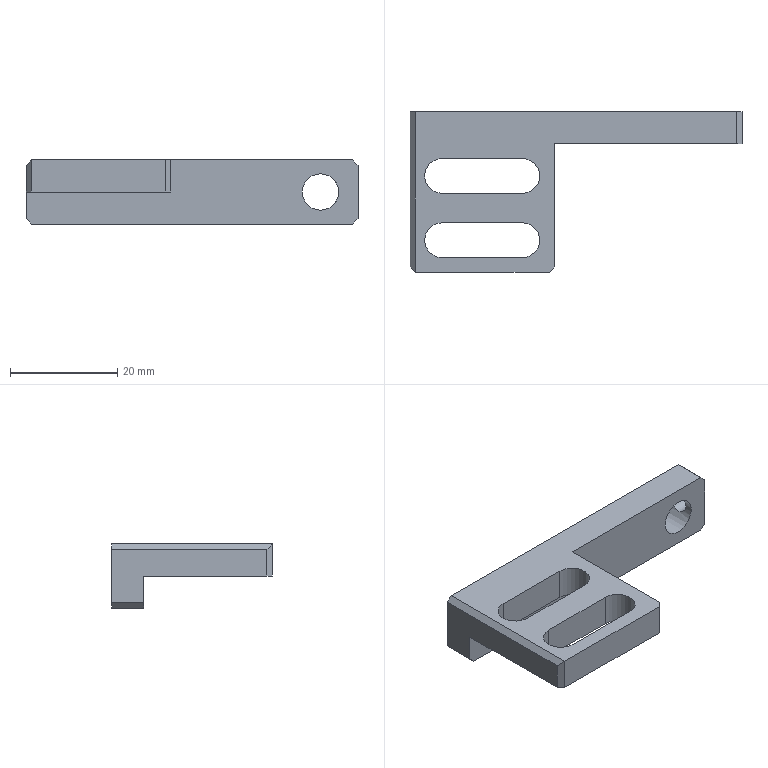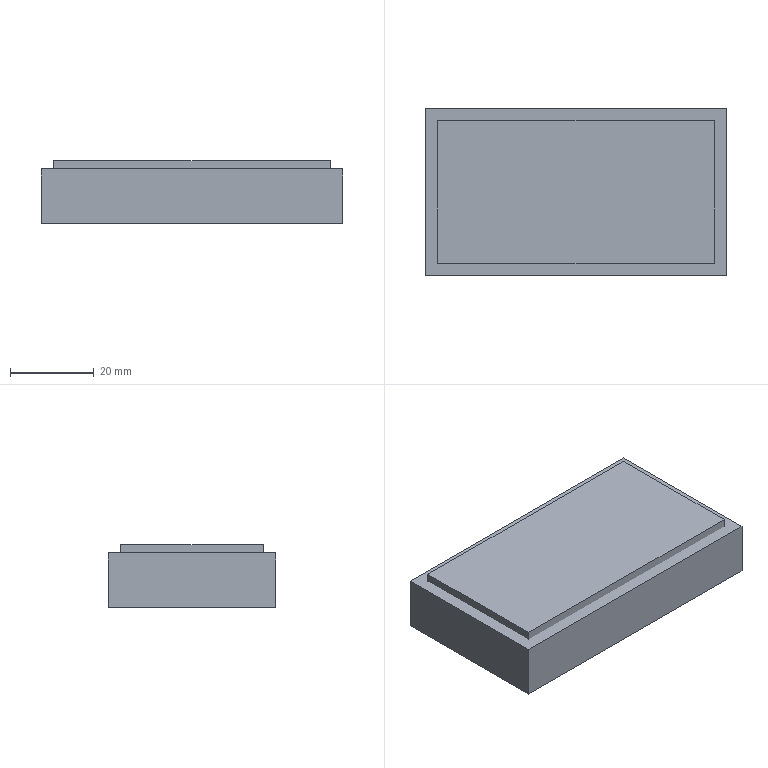CAM job | NX | 3-axis milling | part box 62 x 30 x 12 mm | stock box 72 x 40 x 15 mm
Tools:
number,name,description,diameter,corner_radius,flute_length,length,flutes
19,D80,Milling Tool-5 Parameters,80.0,0.0,50.0,75.0,2
15,D10,Milling Tool-5 Parameters,10.0,0.0,50.0,75.0,2
14,D10JING,Milling Tool-5 Parameters,10.0,0.0,50.0,75.0,2
11,D4,Milling Tool-5 Parameters,4.0,0.0,50.0,75.0,2
1,D6A45,Milling Tool-5 Parameters,6.0,0.0,50.0,75.0,2
Operations:
program,operation,operation_type,tool,method,geometry_group,spindle_rpm,surface_speed,feed_per_tooth,feed_cut,feed_plunge,cut_length_mm,path_length_mm,cut_time_min,machine_time_min
1,FLOOR_WALL,VolumeBased25DMillingOperation,D80,METHOD,A,6500.0,1633.0,0.1154,1500.0,100.0,164.0,218.0,0.1093,0.1147
1,ADAPTIVE_MILLING,CavityMilling,D10,METHOD,A,9500.0,298.0,0.1579,3000.0,1000.0,3960.182,4038.182,1.322,1.33
1,FLOOR_WALL_1,VolumeBased25DMillingOperation,D10,METHOD,A,9500.0,298.0,0.1579,3000.0,1000.0,1389.879,1455.679,0.4681,0.4747
1,ZLEVEL_PROFILE_COPY_1_COPY,ZLevelMilling,D10JING,METHOD,A,9500.0,298.0,0.0632,1200.0,1000.0,220.09,300.09,0.1843,0.1923
1,FLOOR_WALL_1_COPY,VolumeBased25DMillingOperation,D10JING,METHOD,A,9500.0,298.0,0.0789,1500.0,1000.0,269.999,445.103,0.184,0.2015
1,ZLEVEL_PROFILE,ZLevelMilling,D4,METHOD,A,9500.0,119.0,0.0789,1500.0,100.0,1453.278,1616.694,0.9689,0.9852
1,PLANAR_MILL_COPY_COPY_COPY,PlanarMilling,D6A45,METHOD,A,9500.0,179.0,0.0658,1250.0,100.0,146.749,205.749,0.1174,0.1233
1,PLANAR_MILL_COPY_COPY_COPY_COPY,PlanarMilling,D6A45,METHOD,A,9500.0,179.0,0.0658,1250.0,100.0,179.246,423.487,0.1434,0.1678
2,FLOOR_WALL_COPY,VolumeBased25DMillingOperation,D80,METHOD,B,6500.0,1633.0,0.1154,1500.0,100.0,474.0,934.001,0.316,0.362
2,PLANAR_MILL_COPY_COPY_COPY_COPY_1,PlanarMilling,D6A45,METHOD,B,9500.0,179.0,0.0658,1250.0,100.0,292.911,506.579,0.2343,0.2557